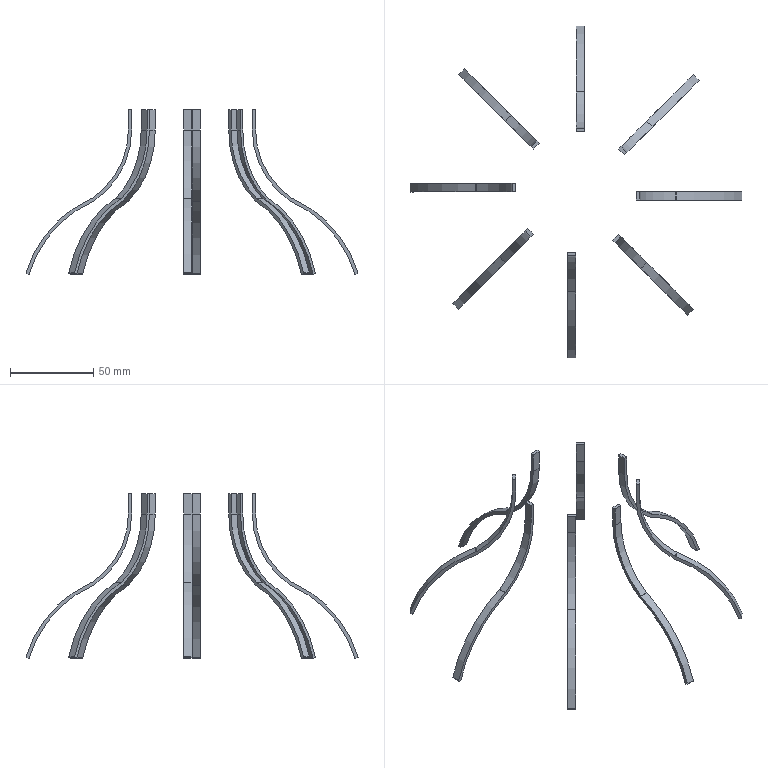Part | SolidWorks | features CirPattern 1, ICE 1 | 8 solids | 120 faces | box 199.946 x 199.946 x 99.301 mm | volume 9875 mm3 | cylinder 72 | plane 48 | commonest cylinder face diameters 1 x40 98.995 x8 102.995 x8 140 x8 144 x8